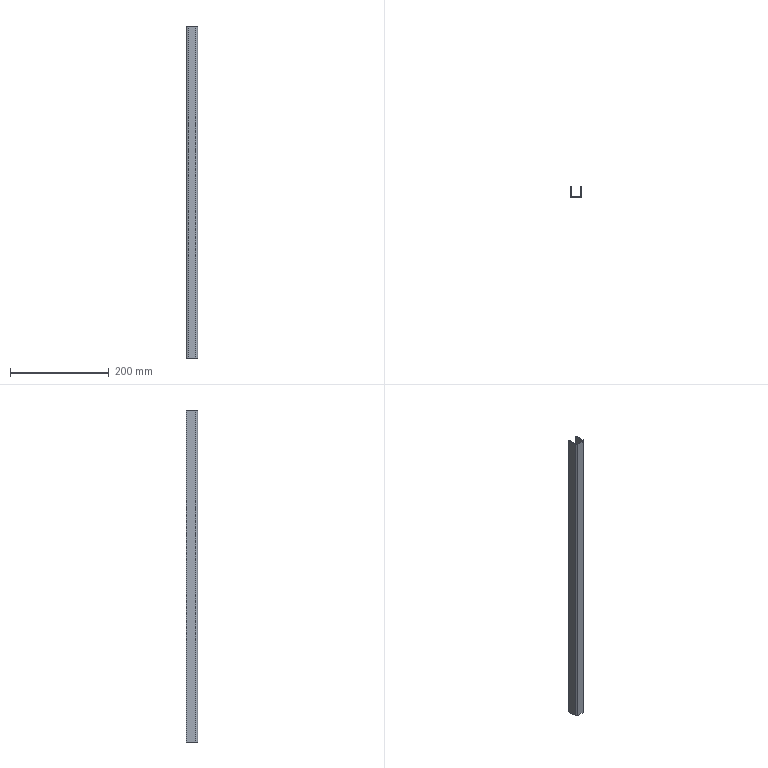Part | NX | features solid 2 | 1 solid | 14 faces | box 23 x 23 x 672 mm | volume 83899 mm3 | plane 10 | cylinder 4 | commonest cylinder face diameters 4 x2 8 x2
STEP:
#1=CARTESIAN_POINT('',(1890.,-671.,1263.));
#2=VERTEX_POINT('',#1);
#3=CARTESIAN_POINT('',(1890.,-652.,1263.));
#4=VERTEX_POINT('',#3);
#5=CARTESIAN_POINT('',(1890.,-675.,1263.));
#6=DIRECTION('',(0.,1.,0.));
#7=VECTOR('',#6,1000.);
#8=LINE('',#5,#7);
#9=EDGE_CURVE('',#2,#4,#8,.T.);
#10=ORIENTED_EDGE('',*,*,#9,.T.);
#11=CARTESIAN_POINT('',(1890.,-652.,591.));
#12=VERTEX_POINT('',#11);
#13=CARTESIAN_POINT('',(1890.,-652.,591.));
#14=DIRECTION('',(0.,0.,1.));
#15=VECTOR('',#14,1000.);
#16=LINE('',#13,#15);
#17=EDGE_CURVE('',#12,#4,#16,.T.);
#18=ORIENTED_EDGE('',*,*,#17,.F.);
#19=CARTESIAN_POINT('',(1890.,-671.,591.));
#20=VERTEX_POINT('',#19);
#21=CARTESIAN_POINT('',(1890.,-675.,591.));
#22=DIRECTION('',(0.,1.,0.));
#23=VECTOR('',#22,1000.);
#24=LINE('',#21,#23);
#25=EDGE_CURVE('',#20,#12,#24,.T.);
#26=ORIENTED_EDGE('',*,*,#25,.F.);
#27=CARTESIAN_POINT('',(1890.,-671.,591.));
#28=DIRECTION('',(0.,0.,1.));
#29=VECTOR('',#28,1000.);
#30=LINE('',#27,#29);
#31=EDGE_CURVE('',#20,#2,#30,.T.);
#32=ORIENTED_EDGE('',*,*,#31,.T.);
#33=EDGE_LOOP('',(#10,#18,#26,#32));
#34=FACE_BOUND('',#33,.T.);
#35=CARTESIAN_POINT('',(1890.,-675.,591.));
#36=DIRECTION('',(1.,0.,0.));
#37=DIRECTION('',(0.,0.,1.));
#38=AXIS2_PLACEMENT_3D('',#35,#36,#37);
#39=PLANE('',#38);
#40=ADVANCED_FACE('',(#34),#39,.F.);
#41=CARTESIAN_POINT('',(1894.,-675.,1263.));
#42=VERTEX_POINT('',#41);
#43=CARTESIAN_POINT('',(1894.,-671.,1263.));
#44=DIRECTION('',(0.,0.,-1.));
#45=DIRECTION('',(0.,-1.,0.));
#46=AXIS2_PLACEMENT_3D('',#43,#44,#45);
#47=CIRCLE('',#46,4.);
#48=EDGE_CURVE('',#42,#2,#47,.T.);
#49=ORIENTED_EDGE('',*,*,#48,.T.);
#50=ORIENTED_EDGE('',*,*,#31,.F.);
#51=CARTESIAN_POINT('',(1894.,-675.,591.));
#52=VERTEX_POINT('',#51);
#53=CARTESIAN_POINT('',(1894.,-671.,591.));
#54=DIRECTION('',(0.,0.,-1.));
#55=DIRECTION('',(0.,-1.,0.));
#56=AXIS2_PLACEMENT_3D('',#53,#54,#55);
#57=CIRCLE('',#56,4.);
#58=EDGE_CURVE('',#52,#20,#57,.T.);
#59=ORIENTED_EDGE('',*,*,#58,.F.);
#60=CARTESIAN_POINT('',(1894.,-675.,591.));
#61=DIRECTION('',(0.,0.,1.));
#62=VECTOR('',#61,1000.);
#63=LINE('',#60,#62);
#64=EDGE_CURVE('',#52,#42,#63,.T.);
#65=ORIENTED_EDGE('',*,*,#64,.T.);
#66=EDGE_LOOP('',(#49,#50,#59,#65));
#67=FACE_BOUND('',#66,.T.);
#68=CARTESIAN_POINT('',(1894.,-671.,591.));
#69=DIRECTION('',(0.,0.,1.));
#70=DIRECTION('',(0.,-1.,0.));
#71=AXIS2_PLACEMENT_3D('',#68,#69,#70);
#72=CYLINDRICAL_SURFACE('',#71,4.);
#73=ADVANCED_FACE('',(#67),#72,.T.);
#74=CARTESIAN_POINT('',(1909.,-675.,1263.));
#75=VERTEX_POINT('',#74);
#76=CARTESIAN_POINT('',(1913.,-675.,1263.));
#77=DIRECTION('',(-1.,0.,0.));
#78=VECTOR('',#77,1000.);
#79=LINE('',#76,#78);
#80=EDGE_CURVE('',#75,#42,#79,.T.);
#81=ORIENTED_EDGE('',*,*,#80,.T.);
#82=ORIENTED_EDGE('',*,*,#64,.F.);
#83=CARTESIAN_POINT('',(1909.,-675.,591.));
#84=VERTEX_POINT('',#83);
#85=CARTESIAN_POINT('',(1913.,-675.,591.));
#86=DIRECTION('',(-1.,0.,0.));
#87=VECTOR('',#86,1000.);
#88=LINE('',#85,#87);
#89=EDGE_CURVE('',#84,#52,#88,.T.);
#90=ORIENTED_EDGE('',*,*,#89,.F.);
#91=CARTESIAN_POINT('',(1909.,-675.,591.));
#92=DIRECTION('',(0.,0.,1.));
#93=VECTOR('',#92,1000.);
#94=LINE('',#91,#93);
#95=EDGE_CURVE('',#84,#75,#94,.T.);
#96=ORIENTED_EDGE('',*,*,#95,.T.);
#97=EDGE_LOOP('',(#81,#82,#90,#96));
#98=FACE_BOUND('',#97,.T.);
#99=CARTESIAN_POINT('',(1913.,-675.,591.));
#100=DIRECTION('',(0.,1.,0.));
#101=DIRECTION('',(0.,0.,-1.));
#102=AXIS2_PLACEMENT_3D('',#99,#100,#101);
#103=PLANE('',#102);
#104=ADVANCED_FACE('',(#98),#103,.F.);
#105=CARTESIAN_POINT('',(1913.,-671.,1263.));
#106=VERTEX_POINT('',#105);
#107=CARTESIAN_POINT('',(1909.,-671.,1263.));
#108=DIRECTION('',(0.,0.,-1.));
#109=DIRECTION('',(0.,-1.,0.));
#110=AXIS2_PLACEMENT_3D('',#107,#108,#109);
#111=CIRCLE('',#110,4.);
#112=EDGE_CURVE('',#106,#75,#111,.T.);
#113=ORIENTED_EDGE('',*,*,#112,.T.);
#114=ORIENTED_EDGE('',*,*,#95,.F.);
#115=CARTESIAN_POINT('',(1913.,-671.,591.));
#116=VERTEX_POINT('',#115);
#117=CARTESIAN_POINT('',(1909.,-671.,591.));
#118=DIRECTION('',(0.,0.,-1.));
#119=DIRECTION('',(0.,-1.,0.));
#120=AXIS2_PLACEMENT_3D('',#117,#118,#119);
#121=CIRCLE('',#120,4.);
#122=EDGE_CURVE('',#116,#84,#121,.T.);
#123=ORIENTED_EDGE('',*,*,#122,.F.);
#124=CARTESIAN_POINT('',(1913.,-671.,591.));
#125=DIRECTION('',(0.,0.,1.));
#126=VECTOR('',#125,1000.);
#127=LINE('',#124,#126);
#128=EDGE_CURVE('',#116,#106,#127,.T.);
#129=ORIENTED_EDGE('',*,*,#128,.T.);
#130=EDGE_LOOP('',(#113,#114,#123,#129));
#131=FACE_BOUND('',#130,.T.);
#132=CARTESIAN_POINT('',(1909.,-671.,591.));
#133=DIRECTION('',(0.,0.,1.));
#134=DIRECTION('',(0.,-1.,0.));
#135=AXIS2_PLACEMENT_3D('',#132,#133,#134);
#136=CYLINDRICAL_SURFACE('',#135,4.);
#137=ADVANCED_FACE('',(#131),#136,.T.);
#138=CARTESIAN_POINT('',(1913.,-652.,1263.));
#139=VERTEX_POINT('',#138);
#140=CARTESIAN_POINT('',(1913.,-652.,1263.));
#141=DIRECTION('',(0.,-1.,0.));
#142=VECTOR('',#141,1000.);
#143=LINE('',#140,#142);
#144=EDGE_CURVE('',#139,#106,#143,.T.);
#145=ORIENTED_EDGE('',*,*,#144,.T.);
#146=ORIENTED_EDGE('',*,*,#128,.F.);
#147=CARTESIAN_POINT('',(1913.,-652.,591.));
#148=VERTEX_POINT('',#147);
#149=CARTESIAN_POINT('',(1913.,-652.,591.));
#150=DIRECTION('',(0.,-1.,0.));
#151=VECTOR('',#150,1000.);
#152=LINE('',#149,#151);
#153=EDGE_CURVE('',#148,#116,#152,.T.);
#154=ORIENTED_EDGE('',*,*,#153,.F.);
#155=CARTESIAN_POINT('',(1913.,-652.,591.));
#156=DIRECTION('',(0.,0.,1.));
#157=VECTOR('',#156,1000.);
#158=LINE('',#155,#157);
#159=EDGE_CURVE('',#148,#139,#158,.T.);
#160=ORIENTED_EDGE('',*,*,#159,.T.);
#161=EDGE_LOOP('',(#145,#146,#154,#160));
#162=FACE_BOUND('',#161,.T.);
#163=CARTESIAN_POINT('',(1913.,-652.,591.));
#164=DIRECTION('',(-1.,0.,0.));
#165=DIRECTION('',(0.,0.,1.));
#166=AXIS2_PLACEMENT_3D('',#163,#164,#165);
#167=PLANE('',#166);
#168=ADVANCED_FACE('',(#162),#167,.F.);
#169=CARTESIAN_POINT('',(1892.,-671.,1263.));
#170=VERTEX_POINT('',#169);
#171=CARTESIAN_POINT('',(1892.,-652.,1263.));
#172=VERTEX_POINT('',#171);
#173=CARTESIAN_POINT('',(1892.,-675.,1263.));
#174=DIRECTION('',(0.,1.,0.));
#175=VECTOR('',#174,1000.);
#176=LINE('',#173,#175);
#177=EDGE_CURVE('',#170,#172,#176,.T.);
#178=ORIENTED_EDGE('',*,*,#177,.F.);
#179=CARTESIAN_POINT('',(1892.,-671.,591.));
#180=VERTEX_POINT('',#179);
#181=CARTESIAN_POINT('',(1892.,-671.,591.));
#182=DIRECTION('',(0.,0.,1.));
#183=VECTOR('',#182,1000.);
#184=LINE('',#181,#183);
#185=EDGE_CURVE('',#180,#170,#184,.T.);
#186=ORIENTED_EDGE('',*,*,#185,.F.);
#187=CARTESIAN_POINT('',(1892.,-652.,591.));
#188=VERTEX_POINT('',#187);
#189=CARTESIAN_POINT('',(1892.,-675.,591.));
#190=DIRECTION('',(0.,1.,0.));
#191=VECTOR('',#190,1000.);
#192=LINE('',#189,#191);
#193=EDGE_CURVE('',#180,#188,#192,.T.);
#194=ORIENTED_EDGE('',*,*,#193,.T.);
#195=CARTESIAN_POINT('',(1892.,-652.,591.));
#196=DIRECTION('',(0.,0.,1.));
#197=VECTOR('',#196,1000.);
#198=LINE('',#195,#197);
#199=EDGE_CURVE('',#188,#172,#198,.T.);
#200=ORIENTED_EDGE('',*,*,#199,.T.);
#201=EDGE_LOOP('',(#178,#186,#194,#200));
#202=FACE_BOUND('',#201,.T.);
#203=CARTESIAN_POINT('',(1892.,-675.,591.));
#204=DIRECTION('',(1.,0.,0.));
#205=DIRECTION('',(0.,0.,1.));
#206=AXIS2_PLACEMENT_3D('',#203,#204,#205);
#207=PLANE('',#206);
#208=ADVANCED_FACE('',(#202),#207,.T.);
#209=CARTESIAN_POINT('',(1894.,-673.,1263.));
#210=VERTEX_POINT('',#209);
#211=CARTESIAN_POINT('',(1894.,-671.,1263.));
#212=DIRECTION('',(0.,0.,-1.));
#213=DIRECTION('',(0.,-1.,0.));
#214=AXIS2_PLACEMENT_3D('',#211,#212,#213);
#215=CIRCLE('',#214,2.);
#216=EDGE_CURVE('',#210,#170,#215,.T.);
#217=ORIENTED_EDGE('',*,*,#216,.F.);
#218=CARTESIAN_POINT('',(1894.,-673.,591.));
#219=VERTEX_POINT('',#218);
#220=CARTESIAN_POINT('',(1894.,-673.,591.));
#221=DIRECTION('',(0.,0.,1.));
#222=VECTOR('',#221,1000.);
#223=LINE('',#220,#222);
#224=EDGE_CURVE('',#219,#210,#223,.T.);
#225=ORIENTED_EDGE('',*,*,#224,.F.);
#226=CARTESIAN_POINT('',(1894.,-671.,591.));
#227=DIRECTION('',(0.,0.,-1.));
#228=DIRECTION('',(0.,-1.,0.));
#229=AXIS2_PLACEMENT_3D('',#226,#227,#228);
#230=CIRCLE('',#229,2.);
#231=EDGE_CURVE('',#219,#180,#230,.T.);
#232=ORIENTED_EDGE('',*,*,#231,.T.);
#233=ORIENTED_EDGE('',*,*,#185,.T.);
#234=EDGE_LOOP('',(#217,#225,#232,#233));
#235=FACE_BOUND('',#234,.T.);
#236=CARTESIAN_POINT('',(1894.,-671.,591.));
#237=DIRECTION('',(0.,0.,1.));
#238=DIRECTION('',(0.,-1.,0.));
#239=AXIS2_PLACEMENT_3D('',#236,#237,#238);
#240=CYLINDRICAL_SURFACE('',#239,2.);
#241=ADVANCED_FACE('',(#235),#240,.F.);
#242=CARTESIAN_POINT('',(1909.,-673.,1263.));
#243=VERTEX_POINT('',#242);
#244=CARTESIAN_POINT('',(1913.,-673.,1263.));
#245=DIRECTION('',(-1.,0.,0.));
#246=VECTOR('',#245,1000.);
#247=LINE('',#244,#246);
#248=EDGE_CURVE('',#243,#210,#247,.T.);
#249=ORIENTED_EDGE('',*,*,#248,.F.);
#250=CARTESIAN_POINT('',(1909.,-673.,591.));
#251=VERTEX_POINT('',#250);
#252=CARTESIAN_POINT('',(1909.,-673.,591.));
#253=DIRECTION('',(0.,0.,1.));
#254=VECTOR('',#253,1000.);
#255=LINE('',#252,#254);
#256=EDGE_CURVE('',#251,#243,#255,.T.);
#257=ORIENTED_EDGE('',*,*,#256,.F.);
#258=CARTESIAN_POINT('',(1913.,-673.,591.));
#259=DIRECTION('',(-1.,0.,0.));
#260=VECTOR('',#259,1000.);
#261=LINE('',#258,#260);
#262=EDGE_CURVE('',#251,#219,#261,.T.);
#263=ORIENTED_EDGE('',*,*,#262,.T.);
#264=ORIENTED_EDGE('',*,*,#224,.T.);
#265=EDGE_LOOP('',(#249,#257,#263,#264));
#266=FACE_BOUND('',#265,.T.);
#267=CARTESIAN_POINT('',(1913.,-673.,591.));
#268=DIRECTION('',(0.,1.,0.));
#269=DIRECTION('',(0.,0.,-1.));
#270=AXIS2_PLACEMENT_3D('',#267,#268,#269);
#271=PLANE('',#270);
#272=ADVANCED_FACE('',(#266),#271,.T.);
#273=CARTESIAN_POINT('',(1911.,-671.,1263.));
#274=VERTEX_POINT('',#273);
#275=CARTESIAN_POINT('',(1909.,-671.,1263.));
#276=DIRECTION('',(0.,0.,-1.));
#277=DIRECTION('',(0.,-1.,0.));
#278=AXIS2_PLACEMENT_3D('',#275,#276,#277);
#279=CIRCLE('',#278,2.);
#280=EDGE_CURVE('',#274,#243,#279,.T.);
#281=ORIENTED_EDGE('',*,*,#280,.F.);
#282=CARTESIAN_POINT('',(1911.,-671.,591.));
#283=VERTEX_POINT('',#282);
#284=CARTESIAN_POINT('',(1911.,-671.,591.));
#285=DIRECTION('',(0.,0.,1.));
#286=VECTOR('',#285,1000.);
#287=LINE('',#284,#286);
#288=EDGE_CURVE('',#283,#274,#287,.T.);
#289=ORIENTED_EDGE('',*,*,#288,.F.);
#290=CARTESIAN_POINT('',(1909.,-671.,591.));
#291=DIRECTION('',(0.,0.,-1.));
#292=DIRECTION('',(0.,-1.,0.));
#293=AXIS2_PLACEMENT_3D('',#290,#291,#292);
#294=CIRCLE('',#293,2.);
#295=EDGE_CURVE('',#283,#251,#294,.T.);
#296=ORIENTED_EDGE('',*,*,#295,.T.);
#297=ORIENTED_EDGE('',*,*,#256,.T.);
#298=EDGE_LOOP('',(#281,#289,#296,#297));
#299=FACE_BOUND('',#298,.T.);
#300=CARTESIAN_POINT('',(1909.,-671.,591.));
#301=DIRECTION('',(0.,0.,1.));
#302=DIRECTION('',(0.,-1.,0.));
#303=AXIS2_PLACEMENT_3D('',#300,#301,#302);
#304=CYLINDRICAL_SURFACE('',#303,2.);
#305=ADVANCED_FACE('',(#299),#304,.F.);
#306=CARTESIAN_POINT('',(1911.,-652.,1263.));
#307=VERTEX_POINT('',#306);
#308=CARTESIAN_POINT('',(1911.,-652.,1263.));
#309=DIRECTION('',(0.,-1.,0.));
#310=VECTOR('',#309,1000.);
#311=LINE('',#308,#310);
#312=EDGE_CURVE('',#307,#274,#311,.T.);
#313=ORIENTED_EDGE('',*,*,#312,.F.);
#314=CARTESIAN_POINT('',(1911.,-652.,591.));
#315=VERTEX_POINT('',#314);
#316=CARTESIAN_POINT('',(1911.,-652.,591.));
#317=DIRECTION('',(0.,0.,1.));
#318=VECTOR('',#317,1000.);
#319=LINE('',#316,#318);
#320=EDGE_CURVE('',#315,#307,#319,.T.);
#321=ORIENTED_EDGE('',*,*,#320,.F.);
#322=CARTESIAN_POINT('',(1911.,-652.,591.));
#323=DIRECTION('',(0.,-1.,0.));
#324=VECTOR('',#323,1000.);
#325=LINE('',#322,#324);
#326=EDGE_CURVE('',#315,#283,#325,.T.);
#327=ORIENTED_EDGE('',*,*,#326,.T.);
#328=ORIENTED_EDGE('',*,*,#288,.T.);
#329=EDGE_LOOP('',(#313,#321,#327,#328));
#330=FACE_BOUND('',#329,.T.);
#331=CARTESIAN_POINT('',(1911.,-652.,591.));
#332=DIRECTION('',(-1.,0.,0.));
#333=DIRECTION('',(0.,0.,1.));
#334=AXIS2_PLACEMENT_3D('',#331,#332,#333);
#335=PLANE('',#334);
#336=ADVANCED_FACE('',(#330),#335,.T.);
#337=ORIENTED_EDGE('',*,*,#159,.F.);
#338=CARTESIAN_POINT('',(1913.,-652.,591.));
#339=DIRECTION('',(-1.,0.,0.));
#340=VECTOR('',#339,1000.);
#341=LINE('',#338,#340);
#342=EDGE_CURVE('',#148,#315,#341,.T.);
#343=ORIENTED_EDGE('',*,*,#342,.T.);
#344=ORIENTED_EDGE('',*,*,#320,.T.);
#345=CARTESIAN_POINT('',(1913.,-652.,1263.));
#346=DIRECTION('',(-1.,0.,0.));
#347=VECTOR('',#346,1000.);
#348=LINE('',#345,#347);
#349=EDGE_CURVE('',#139,#307,#348,.T.);
#350=ORIENTED_EDGE('',*,*,#349,.F.);
#351=EDGE_LOOP('',(#337,#343,#344,#350));
#352=FACE_BOUND('',#351,.T.);
#353=CARTESIAN_POINT('',(1913.,-652.,591.));
#354=DIRECTION('',(0.,-1.,0.));
#355=DIRECTION('',(-1.,0.,0.));
#356=AXIS2_PLACEMENT_3D('',#353,#354,#355);
#357=PLANE('',#356);
#358=ADVANCED_FACE('',(#352),#357,.F.);
#359=ORIENTED_EDGE('',*,*,#312,.T.);
#360=ORIENTED_EDGE('',*,*,#280,.T.);
#361=ORIENTED_EDGE('',*,*,#248,.T.);
#362=ORIENTED_EDGE('',*,*,#216,.T.);
#363=ORIENTED_EDGE('',*,*,#177,.T.);
#364=CARTESIAN_POINT('',(1890.,-652.,1263.));
#365=DIRECTION('',(1.,0.,0.));
#366=VECTOR('',#365,1000.);
#367=LINE('',#364,#366);
#368=EDGE_CURVE('',#4,#172,#367,.T.);
#369=ORIENTED_EDGE('',*,*,#368,.F.);
#370=ORIENTED_EDGE('',*,*,#9,.F.);
#371=ORIENTED_EDGE('',*,*,#48,.F.);
#372=ORIENTED_EDGE('',*,*,#80,.F.);
#373=ORIENTED_EDGE('',*,*,#112,.F.);
#374=ORIENTED_EDGE('',*,*,#144,.F.);
#375=ORIENTED_EDGE('',*,*,#349,.T.);
#376=EDGE_LOOP('',(#359,#360,#361,#362,#363,#369,#370,#371,#372,#373,#374,#375));
#377=FACE_BOUND('',#376,.T.);
#378=CARTESIAN_POINT('',(1913.,-652.,1263.));
#379=DIRECTION('',(0.,0.,-1.));
#380=DIRECTION('',(0.,-1.,0.));
#381=AXIS2_PLACEMENT_3D('',#378,#379,#380);
#382=PLANE('',#381);
#383=ADVANCED_FACE('',(#377),#382,.F.);
#384=CARTESIAN_POINT('',(1890.,-652.,591.));
#385=DIRECTION('',(1.,0.,0.));
#386=VECTOR('',#385,1000.);
#387=LINE('',#384,#386);
#388=EDGE_CURVE('',#12,#188,#387,.T.);
#389=ORIENTED_EDGE('',*,*,#388,.F.);
#390=ORIENTED_EDGE('',*,*,#17,.T.);
#391=ORIENTED_EDGE('',*,*,#368,.T.);
#392=ORIENTED_EDGE('',*,*,#199,.F.);
#393=EDGE_LOOP('',(#389,#390,#391,#392));
#394=FACE_BOUND('',#393,.T.);
#395=CARTESIAN_POINT('',(1890.,-652.,591.));
#396=DIRECTION('',(0.,1.,0.));
#397=DIRECTION('',(0.,0.,-1.));
#398=AXIS2_PLACEMENT_3D('',#395,#396,#397);
#399=PLANE('',#398);
#400=ADVANCED_FACE('',(#394),#399,.T.);
#401=ORIENTED_EDGE('',*,*,#193,.F.);
#402=ORIENTED_EDGE('',*,*,#231,.F.);
#403=ORIENTED_EDGE('',*,*,#262,.F.);
#404=ORIENTED_EDGE('',*,*,#295,.F.);
#405=ORIENTED_EDGE('',*,*,#326,.F.);
#406=ORIENTED_EDGE('',*,*,#342,.F.);
#407=ORIENTED_EDGE('',*,*,#153,.T.);
#408=ORIENTED_EDGE('',*,*,#122,.T.);
#409=ORIENTED_EDGE('',*,*,#89,.T.);
#410=ORIENTED_EDGE('',*,*,#58,.T.);
#411=ORIENTED_EDGE('',*,*,#25,.T.);
#412=ORIENTED_EDGE('',*,*,#388,.T.);
#413=EDGE_LOOP('',(#401,#402,#403,#404,#405,#406,#407,#408,#409,#410,#411,#412));
#414=FACE_BOUND('',#413,.T.);
#415=CARTESIAN_POINT('',(1890.,-675.,591.));
#416=DIRECTION('',(0.,0.,-1.));
#417=DIRECTION('',(0.,-1.,0.));
#418=AXIS2_PLACEMENT_3D('',#415,#416,#417);
#419=PLANE('',#418);
#420=ADVANCED_FACE('',(#414),#419,.T.);
#421=CLOSED_SHELL('',(#40,#73,#104,#137,#168,#208,#241,#272,#305,#336,#358,#383,#400,#420));
#422=MANIFOLD_SOLID_BREP('',#421);
#423=(LENGTH_UNIT()NAMED_UNIT(*)SI_UNIT(.MILLI.,.METRE.));
#424=UNCERTAINTY_MEASURE_WITH_UNIT(LENGTH_MEASURE(0.00001),#423,'','');
#425=(NAMED_UNIT(*)PLANE_ANGLE_UNIT()SI_UNIT($,.RADIAN.));
#426=(NAMED_UNIT(*)SI_UNIT($,.STERADIAN.)SOLID_ANGLE_UNIT());
#427=(GEOMETRIC_REPRESENTATION_CONTEXT(3)GLOBAL_UNCERTAINTY_ASSIGNED_CONTEXT((#424))GLOBAL_UNIT_ASSIGNED_CONTEXT((#423,#425,#426))REPRESENTATION_CONTEXT('',''));
#428=ADVANCED_BREP_SHAPE_REPRESENTATION('',(#422),#427);